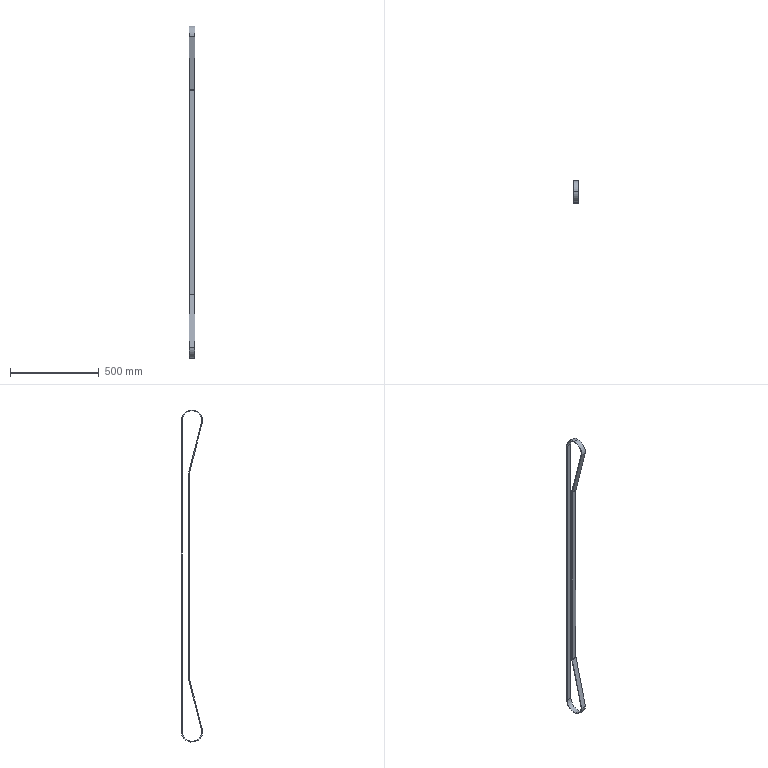Part | SolidWorks | features ExtruThin 1 | 1 solid | 20 faces | box 30 x 121.59 x 1872 mm | volume 524754 mm3 | cylinder 10 | plane 10 | commonest cylinder face diameters 112.59 x3 121.59 x3 37 x2 46 x2
STEP:
#1=CARTESIAN_POINT('',(15.,56.295,1750.));
#2=VERTEX_POINT('',#1);
#3=CARTESIAN_POINT('',(15.,0.,1806.295));
#4=VERTEX_POINT('',#3);
#5=CARTESIAN_POINT('',(15.,0.,1750.));
#6=DIRECTION('',(1.,0.,0.));
#7=DIRECTION('',(0.,0.,-1.));
#8=AXIS2_PLACEMENT_3D('',#5,#6,#7);
#9=CIRCLE('',#8,56.295);
#10=EDGE_CURVE('',#2,#4,#9,.T.);
#11=ORIENTED_EDGE('',*,*,#10,.T.);
#12=CARTESIAN_POINT('',(-15.,0.,1806.295));
#13=VERTEX_POINT('',#12);
#14=CARTESIAN_POINT('',(15.,0.,1806.295));
#15=DIRECTION('',(-1.,0.,0.));
#16=VECTOR('',#15,1000.);
#17=LINE('',#14,#16);
#18=EDGE_CURVE('',#4,#13,#17,.T.);
#19=ORIENTED_EDGE('',*,*,#18,.T.);
#20=CARTESIAN_POINT('',(-15.,56.295,1750.));
#21=VERTEX_POINT('',#20);
#22=CARTESIAN_POINT('',(-15.,0.,1750.));
#23=DIRECTION('',(1.,0.,0.));
#24=DIRECTION('',(0.,0.,-1.));
#25=AXIS2_PLACEMENT_3D('',#22,#23,#24);
#26=CIRCLE('',#25,56.295);
#27=EDGE_CURVE('',#21,#13,#26,.T.);
#28=ORIENTED_EDGE('',*,*,#27,.F.);
#29=CARTESIAN_POINT('',(15.,56.295,1750.));
#30=DIRECTION('',(-1.,0.,0.));
#31=VECTOR('',#30,1000.);
#32=LINE('',#29,#31);
#33=EDGE_CURVE('',#2,#21,#32,.T.);
#34=ORIENTED_EDGE('',*,*,#33,.F.);
#35=EDGE_LOOP('',(#11,#19,#28,#34));
#36=FACE_OUTER_BOUND('',#35,.T.);
#37=CARTESIAN_POINT('',(15.,0.,1750.));
#38=DIRECTION('',(-1.,0.,0.));
#39=DIRECTION('',(0.,0.,1.));
#40=AXIS2_PLACEMENT_3D('',#37,#38,#39);
#41=CYLINDRICAL_SURFACE('',#40,56.295);
#42=ADVANCED_FACE('',(#36),#41,.F.);
#43=CARTESIAN_POINT('',(15.,0.,1810.795));
#44=VERTEX_POINT('',#43);
#45=CARTESIAN_POINT('',(15.,-60.793,1749.552));
#46=VERTEX_POINT('',#45);
#47=CARTESIAN_POINT('',(15.,0.,1750.));
#48=DIRECTION('',(1.,0.,0.));
#49=DIRECTION('',(0.,0.,-1.));
#50=AXIS2_PLACEMENT_3D('',#47,#48,#49);
#51=CIRCLE('',#50,60.795);
#52=EDGE_CURVE('',#44,#46,#51,.T.);
#53=ORIENTED_EDGE('',*,*,#52,.F.);
#54=CARTESIAN_POINT('',(-15.,0.,1810.795));
#55=VERTEX_POINT('',#54);
#56=CARTESIAN_POINT('',(15.,0.,1810.795));
#57=DIRECTION('',(-1.,0.,0.));
#58=VECTOR('',#57,1000.);
#59=LINE('',#56,#58);
#60=EDGE_CURVE('',#44,#55,#59,.T.);
#61=ORIENTED_EDGE('',*,*,#60,.T.);
#62=CARTESIAN_POINT('',(-15.,-60.793,1749.552));
#63=VERTEX_POINT('',#62);
#64=CARTESIAN_POINT('',(-15.,0.,1750.));
#65=DIRECTION('',(1.,0.,0.));
#66=DIRECTION('',(0.,0.,-1.));
#67=AXIS2_PLACEMENT_3D('',#64,#65,#66);
#68=CIRCLE('',#67,60.795);
#69=EDGE_CURVE('',#55,#63,#68,.T.);
#70=ORIENTED_EDGE('',*,*,#69,.T.);
#71=CARTESIAN_POINT('',(15.,-60.793,1749.552));
#72=DIRECTION('',(-1.,0.,0.));
#73=VECTOR('',#72,1000.);
#74=LINE('',#71,#73);
#75=EDGE_CURVE('',#46,#63,#74,.T.);
#76=ORIENTED_EDGE('',*,*,#75,.F.);
#77=EDGE_LOOP('',(#53,#61,#70,#76));
#78=FACE_OUTER_BOUND('',#77,.T.);
#79=CARTESIAN_POINT('',(15.,0.,1750.));
#80=DIRECTION('',(-1.,0.,0.));
#81=DIRECTION('',(0.,0.,1.));
#82=AXIS2_PLACEMENT_3D('',#79,#80,#81);
#83=CYLINDRICAL_SURFACE('',#82,60.795);
#84=ADVANCED_FACE('',(#78),#83,.T.);
#85=CARTESIAN_POINT('',(15.,60.795,1750.));
#86=VERTEX_POINT('',#85);
#87=CARTESIAN_POINT('',(15.,0.,1750.));
#88=DIRECTION('',(1.,0.,0.));
#89=DIRECTION('',(0.,0.,-1.));
#90=AXIS2_PLACEMENT_3D('',#87,#88,#89);
#91=CIRCLE('',#90,60.795);
#92=EDGE_CURVE('',#86,#44,#91,.T.);
#93=ORIENTED_EDGE('',*,*,#92,.T.);
#94=ORIENTED_EDGE('',*,*,#52,.T.);
#95=CARTESIAN_POINT('',(15.,14.914,1454.599));
#96=VERTEX_POINT('',#95);
#97=CARTESIAN_POINT('',(15.,14.914,1454.599));
#98=DIRECTION('',(0.,0.2486,-0.9686));
#99=VECTOR('',#98,1000.);
#100=LINE('',#97,#99);
#101=EDGE_CURVE('',#46,#96,#100,.T.);
#102=ORIENTED_EDGE('',*,*,#101,.T.);
#103=CARTESIAN_POINT('',(15.,15.495,1450.));
#104=VERTEX_POINT('',#103);
#105=CARTESIAN_POINT('',(15.,-3.005,1450.));
#106=DIRECTION('',(-1.,0.,0.));
#107=DIRECTION('',(0.,0.,-1.));
#108=AXIS2_PLACEMENT_3D('',#105,#106,#107);
#109=CIRCLE('',#108,18.5);
#110=EDGE_CURVE('',#96,#104,#109,.T.);
#111=ORIENTED_EDGE('',*,*,#110,.T.);
#112=CARTESIAN_POINT('',(15.,15.495,300.));
#113=VERTEX_POINT('',#112);
#114=CARTESIAN_POINT('',(15.,15.495,1450.));
#115=DIRECTION('',(0.,0.,-1.));
#116=VECTOR('',#115,1000.);
#117=LINE('',#114,#116);
#118=EDGE_CURVE('',#104,#113,#117,.T.);
#119=ORIENTED_EDGE('',*,*,#118,.T.);
#120=CARTESIAN_POINT('',(15.,14.914,295.401));
#121=VERTEX_POINT('',#120);
#122=CARTESIAN_POINT('',(15.,-3.005,300.));
#123=DIRECTION('',(-1.,0.,0.));
#124=DIRECTION('',(0.,0.,-1.));
#125=AXIS2_PLACEMENT_3D('',#122,#123,#124);
#126=CIRCLE('',#125,18.5);
#127=EDGE_CURVE('',#113,#121,#126,.T.);
#128=ORIENTED_EDGE('',*,*,#127,.T.);
#129=CARTESIAN_POINT('',(15.,-60.793,0.4485));
#130=VERTEX_POINT('',#129);
#131=CARTESIAN_POINT('',(15.,-60.685,0.8702));
#132=DIRECTION('',(0.,-0.2486,-0.9686));
#133=VECTOR('',#132,1000.);
#134=LINE('',#131,#133);
#135=EDGE_CURVE('',#121,#130,#134,.T.);
#136=ORIENTED_EDGE('',*,*,#135,.T.);
#137=CARTESIAN_POINT('',(15.,60.795,0.));
#138=VERTEX_POINT('',#137);
#139=CARTESIAN_POINT('',(15.,0.,0.));
#140=DIRECTION('',(1.,0.,0.));
#141=DIRECTION('',(0.,0.,-1.));
#142=AXIS2_PLACEMENT_3D('',#139,#140,#141);
#143=CIRCLE('',#142,60.795);
#144=EDGE_CURVE('',#130,#138,#143,.T.);
#145=ORIENTED_EDGE('',*,*,#144,.T.);
#146=CARTESIAN_POINT('',(15.,60.795,0.));
#147=DIRECTION('',(0.,0.,1.));
#148=VECTOR('',#147,1000.);
#149=LINE('',#146,#148);
#150=EDGE_CURVE('',#138,#86,#149,.T.);
#151=ORIENTED_EDGE('',*,*,#150,.T.);
#152=EDGE_LOOP('',(#93,#94,#102,#111,#119,#128,#136,#145,#151));
#153=FACE_OUTER_BOUND('',#152,.T.);
#154=CARTESIAN_POINT('',(15.,-56.295,1750.126));
#155=VERTEX_POINT('',#154);
#156=CARTESIAN_POINT('',(15.,19.273,1455.718));
#157=VERTEX_POINT('',#156);
#158=CARTESIAN_POINT('',(15.,19.273,1455.718));
#159=DIRECTION('',(0.,0.2486,-0.9686));
#160=VECTOR('',#159,1000.);
#161=LINE('',#158,#160);
#162=EDGE_CURVE('',#155,#157,#161,.T.);
#163=ORIENTED_EDGE('',*,*,#162,.F.);
#164=CARTESIAN_POINT('',(15.,0.,1750.));
#165=DIRECTION('',(1.,0.,0.));
#166=DIRECTION('',(0.,0.,-1.));
#167=AXIS2_PLACEMENT_3D('',#164,#165,#166);
#168=CIRCLE('',#167,56.295);
#169=EDGE_CURVE('',#4,#155,#168,.T.);
#170=ORIENTED_EDGE('',*,*,#169,.F.);
#171=ORIENTED_EDGE('',*,*,#10,.F.);
#172=CARTESIAN_POINT('',(15.,56.295,0.));
#173=VERTEX_POINT('',#172);
#174=CARTESIAN_POINT('',(15.,56.295,0.));
#175=DIRECTION('',(0.,0.,1.));
#176=VECTOR('',#175,1000.);
#177=LINE('',#174,#176);
#178=EDGE_CURVE('',#173,#2,#177,.T.);
#179=ORIENTED_EDGE('',*,*,#178,.F.);
#180=CARTESIAN_POINT('',(15.,-56.295,-0.1257));
#181=VERTEX_POINT('',#180);
#182=CARTESIAN_POINT('',(15.,0.,0.));
#183=DIRECTION('',(1.,0.,0.));
#184=DIRECTION('',(0.,0.,-1.));
#185=AXIS2_PLACEMENT_3D('',#182,#183,#184);
#186=CIRCLE('',#185,56.295);
#187=EDGE_CURVE('',#181,#173,#186,.T.);
#188=ORIENTED_EDGE('',*,*,#187,.F.);
#189=CARTESIAN_POINT('',(15.,19.273,294.282));
#190=VERTEX_POINT('',#189);
#191=CARTESIAN_POINT('',(15.,-56.326,-0.2486));
#192=DIRECTION('',(0.,-0.2486,-0.9686));
#193=VECTOR('',#192,1000.);
#194=LINE('',#191,#193);
#195=EDGE_CURVE('',#190,#181,#194,.T.);
#196=ORIENTED_EDGE('',*,*,#195,.F.);
#197=CARTESIAN_POINT('',(15.,19.995,300.));
#198=VERTEX_POINT('',#197);
#199=CARTESIAN_POINT('',(15.,-3.005,300.));
#200=DIRECTION('',(-1.,0.,0.));
#201=DIRECTION('',(0.,0.,-1.));
#202=AXIS2_PLACEMENT_3D('',#199,#200,#201);
#203=CIRCLE('',#202,23.);
#204=EDGE_CURVE('',#198,#190,#203,.T.);
#205=ORIENTED_EDGE('',*,*,#204,.F.);
#206=CARTESIAN_POINT('',(15.,19.995,1450.));
#207=VERTEX_POINT('',#206);
#208=CARTESIAN_POINT('',(15.,19.995,1450.));
#209=DIRECTION('',(0.,0.,-1.));
#210=VECTOR('',#209,1000.);
#211=LINE('',#208,#210);
#212=EDGE_CURVE('',#207,#198,#211,.T.);
#213=ORIENTED_EDGE('',*,*,#212,.F.);
#214=CARTESIAN_POINT('',(15.,-3.005,1450.));
#215=DIRECTION('',(-1.,0.,0.));
#216=DIRECTION('',(0.,0.,-1.));
#217=AXIS2_PLACEMENT_3D('',#214,#215,#216);
#218=CIRCLE('',#217,23.);
#219=EDGE_CURVE('',#157,#207,#218,.T.);
#220=ORIENTED_EDGE('',*,*,#219,.F.);
#221=EDGE_LOOP('',(#163,#170,#171,#179,#188,#196,#205,#213,#220));
#222=FACE_BOUND('',#221,.T.);
#223=CARTESIAN_POINT('',(15.,0.,1750.));
#224=DIRECTION('',(1.,0.,0.));
#225=DIRECTION('',(0.,0.,-1.));
#226=AXIS2_PLACEMENT_3D('',#223,#224,#225);
#227=PLANE('',#226);
#228=ADVANCED_FACE('',(#153,#222),#227,.T.);
#229=CARTESIAN_POINT('',(-15.,60.795,1750.));
#230=VERTEX_POINT('',#229);
#231=CARTESIAN_POINT('',(-15.,0.,1750.));
#232=DIRECTION('',(1.,0.,0.));
#233=DIRECTION('',(0.,0.,-1.));
#234=AXIS2_PLACEMENT_3D('',#231,#232,#233);
#235=CIRCLE('',#234,60.795);
#236=EDGE_CURVE('',#230,#55,#235,.T.);
#237=ORIENTED_EDGE('',*,*,#236,.F.);
#238=CARTESIAN_POINT('',(-15.,60.795,0.));
#239=VERTEX_POINT('',#238);
#240=CARTESIAN_POINT('',(-15.,60.795,0.));
#241=DIRECTION('',(0.,0.,1.));
#242=VECTOR('',#241,1000.);
#243=LINE('',#240,#242);
#244=EDGE_CURVE('',#239,#230,#243,.T.);
#245=ORIENTED_EDGE('',*,*,#244,.F.);
#246=CARTESIAN_POINT('',(-15.,-60.793,0.4485));
#247=VERTEX_POINT('',#246);
#248=CARTESIAN_POINT('',(-15.,0.,0.));
#249=DIRECTION('',(1.,0.,0.));
#250=DIRECTION('',(0.,0.,-1.));
#251=AXIS2_PLACEMENT_3D('',#248,#249,#250);
#252=CIRCLE('',#251,60.795);
#253=EDGE_CURVE('',#247,#239,#252,.T.);
#254=ORIENTED_EDGE('',*,*,#253,.F.);
#255=CARTESIAN_POINT('',(-15.,14.914,295.401));
#256=VERTEX_POINT('',#255);
#257=CARTESIAN_POINT('',(-15.,-60.685,0.8702));
#258=DIRECTION('',(0.,-0.2486,-0.9686));
#259=VECTOR('',#258,1000.);
#260=LINE('',#257,#259);
#261=EDGE_CURVE('',#256,#247,#260,.T.);
#262=ORIENTED_EDGE('',*,*,#261,.F.);
#263=CARTESIAN_POINT('',(-15.,15.495,300.));
#264=VERTEX_POINT('',#263);
#265=CARTESIAN_POINT('',(-15.,-3.005,300.));
#266=DIRECTION('',(-1.,0.,0.));
#267=DIRECTION('',(0.,0.,-1.));
#268=AXIS2_PLACEMENT_3D('',#265,#266,#267);
#269=CIRCLE('',#268,18.5);
#270=EDGE_CURVE('',#264,#256,#269,.T.);
#271=ORIENTED_EDGE('',*,*,#270,.F.);
#272=CARTESIAN_POINT('',(-15.,15.495,1450.));
#273=VERTEX_POINT('',#272);
#274=CARTESIAN_POINT('',(-15.,15.495,1450.));
#275=DIRECTION('',(0.,0.,-1.));
#276=VECTOR('',#275,1000.);
#277=LINE('',#274,#276);
#278=EDGE_CURVE('',#273,#264,#277,.T.);
#279=ORIENTED_EDGE('',*,*,#278,.F.);
#280=CARTESIAN_POINT('',(-15.,14.914,1454.599));
#281=VERTEX_POINT('',#280);
#282=CARTESIAN_POINT('',(-15.,-3.005,1450.));
#283=DIRECTION('',(-1.,0.,0.));
#284=DIRECTION('',(0.,0.,-1.));
#285=AXIS2_PLACEMENT_3D('',#282,#283,#284);
#286=CIRCLE('',#285,18.5);
#287=EDGE_CURVE('',#281,#273,#286,.T.);
#288=ORIENTED_EDGE('',*,*,#287,.F.);
#289=CARTESIAN_POINT('',(-15.,14.914,1454.599));
#290=DIRECTION('',(0.,0.2486,-0.9686));
#291=VECTOR('',#290,1000.);
#292=LINE('',#289,#291);
#293=EDGE_CURVE('',#63,#281,#292,.T.);
#294=ORIENTED_EDGE('',*,*,#293,.F.);
#295=ORIENTED_EDGE('',*,*,#69,.F.);
#296=EDGE_LOOP('',(#237,#245,#254,#262,#271,#279,#288,#294,#295));
#297=FACE_OUTER_BOUND('',#296,.T.);
#298=ORIENTED_EDGE('',*,*,#27,.T.);
#299=CARTESIAN_POINT('',(-15.,-56.295,1750.126));
#300=VERTEX_POINT('',#299);
#301=CARTESIAN_POINT('',(-15.,0.,1750.));
#302=DIRECTION('',(1.,0.,0.));
#303=DIRECTION('',(0.,0.,-1.));
#304=AXIS2_PLACEMENT_3D('',#301,#302,#303);
#305=CIRCLE('',#304,56.295);
#306=EDGE_CURVE('',#13,#300,#305,.T.);
#307=ORIENTED_EDGE('',*,*,#306,.T.);
#308=CARTESIAN_POINT('',(-15.,19.273,1455.718));
#309=VERTEX_POINT('',#308);
#310=CARTESIAN_POINT('',(-15.,19.273,1455.718));
#311=DIRECTION('',(0.,0.2486,-0.9686));
#312=VECTOR('',#311,1000.);
#313=LINE('',#310,#312);
#314=EDGE_CURVE('',#300,#309,#313,.T.);
#315=ORIENTED_EDGE('',*,*,#314,.T.);
#316=CARTESIAN_POINT('',(-15.,19.995,1450.));
#317=VERTEX_POINT('',#316);
#318=CARTESIAN_POINT('',(-15.,-3.005,1450.));
#319=DIRECTION('',(-1.,0.,0.));
#320=DIRECTION('',(0.,0.,-1.));
#321=AXIS2_PLACEMENT_3D('',#318,#319,#320);
#322=CIRCLE('',#321,23.);
#323=EDGE_CURVE('',#309,#317,#322,.T.);
#324=ORIENTED_EDGE('',*,*,#323,.T.);
#325=CARTESIAN_POINT('',(-15.,19.995,300.));
#326=VERTEX_POINT('',#325);
#327=CARTESIAN_POINT('',(-15.,19.995,1450.));
#328=DIRECTION('',(0.,0.,-1.));
#329=VECTOR('',#328,1000.);
#330=LINE('',#327,#329);
#331=EDGE_CURVE('',#317,#326,#330,.T.);
#332=ORIENTED_EDGE('',*,*,#331,.T.);
#333=CARTESIAN_POINT('',(-15.,19.273,294.282));
#334=VERTEX_POINT('',#333);
#335=CARTESIAN_POINT('',(-15.,-3.005,300.));
#336=DIRECTION('',(-1.,0.,0.));
#337=DIRECTION('',(0.,0.,-1.));
#338=AXIS2_PLACEMENT_3D('',#335,#336,#337);
#339=CIRCLE('',#338,23.);
#340=EDGE_CURVE('',#326,#334,#339,.T.);
#341=ORIENTED_EDGE('',*,*,#340,.T.);
#342=CARTESIAN_POINT('',(-15.,-56.295,-0.1257));
#343=VERTEX_POINT('',#342);
#344=CARTESIAN_POINT('',(-15.,-56.326,-0.2486));
#345=DIRECTION('',(0.,-0.2486,-0.9686));
#346=VECTOR('',#345,1000.);
#347=LINE('',#344,#346);
#348=EDGE_CURVE('',#334,#343,#347,.T.);
#349=ORIENTED_EDGE('',*,*,#348,.T.);
#350=CARTESIAN_POINT('',(-15.,56.295,0.));
#351=VERTEX_POINT('',#350);
#352=CARTESIAN_POINT('',(-15.,0.,0.));
#353=DIRECTION('',(1.,0.,0.));
#354=DIRECTION('',(0.,0.,-1.));
#355=AXIS2_PLACEMENT_3D('',#352,#353,#354);
#356=CIRCLE('',#355,56.295);
#357=EDGE_CURVE('',#343,#351,#356,.T.);
#358=ORIENTED_EDGE('',*,*,#357,.T.);
#359=CARTESIAN_POINT('',(-15.,56.295,0.));
#360=DIRECTION('',(0.,0.,1.));
#361=VECTOR('',#360,1000.);
#362=LINE('',#359,#361);
#363=EDGE_CURVE('',#351,#21,#362,.T.);
#364=ORIENTED_EDGE('',*,*,#363,.T.);
#365=EDGE_LOOP('',(#298,#307,#315,#324,#332,#341,#349,#358,#364));
#366=FACE_BOUND('',#365,.T.);
#367=CARTESIAN_POINT('',(-15.,0.,1750.));
#368=DIRECTION('',(1.,0.,0.));
#369=DIRECTION('',(0.,0.,-1.));
#370=AXIS2_PLACEMENT_3D('',#367,#368,#369);
#371=PLANE('',#370);
#372=ADVANCED_FACE('',(#297,#366),#371,.F.);
#373=ORIENTED_EDGE('',*,*,#60,.F.);
#374=ORIENTED_EDGE('',*,*,#92,.F.);
#375=CARTESIAN_POINT('',(15.,60.795,1750.));
#376=DIRECTION('',(-1.,0.,0.));
#377=VECTOR('',#376,1000.);
#378=LINE('',#375,#377);
#379=EDGE_CURVE('',#86,#230,#378,.T.);
#380=ORIENTED_EDGE('',*,*,#379,.T.);
#381=ORIENTED_EDGE('',*,*,#236,.T.);
#382=EDGE_LOOP('',(#373,#374,#380,#381));
#383=FACE_OUTER_BOUND('',#382,.T.);
#384=CARTESIAN_POINT('',(15.,0.,1750.));
#385=DIRECTION('',(-1.,0.,0.));
#386=DIRECTION('',(0.,0.,1.));
#387=AXIS2_PLACEMENT_3D('',#384,#385,#386);
#388=CYLINDRICAL_SURFACE('',#387,60.795);
#389=ADVANCED_FACE('',(#383),#388,.T.);
#390=ORIENTED_EDGE('',*,*,#293,.T.);
#391=CARTESIAN_POINT('',(15.,14.914,1454.599));
#392=DIRECTION('',(-1.,0.,0.));
#393=VECTOR('',#392,1000.);
#394=LINE('',#391,#393);
#395=EDGE_CURVE('',#96,#281,#394,.T.);
#396=ORIENTED_EDGE('',*,*,#395,.F.);
#397=ORIENTED_EDGE('',*,*,#101,.F.);
#398=ORIENTED_EDGE('',*,*,#75,.T.);
#399=EDGE_LOOP('',(#390,#396,#397,#398));
#400=FACE_OUTER_BOUND('',#399,.T.);
#401=CARTESIAN_POINT('',(15.,14.914,1454.599));
#402=DIRECTION('',(0.,0.9686,0.2486));
#403=DIRECTION('',(0.,-0.2486,0.9686));
#404=AXIS2_PLACEMENT_3D('',#401,#402,#403);
#405=PLANE('',#404);
#406=ADVANCED_FACE('',(#400),#405,.F.);
#407=ORIENTED_EDGE('',*,*,#287,.T.);
#408=CARTESIAN_POINT('',(15.,15.495,1450.));
#409=DIRECTION('',(-1.,0.,0.));
#410=VECTOR('',#409,1000.);
#411=LINE('',#408,#410);
#412=EDGE_CURVE('',#104,#273,#411,.T.);
#413=ORIENTED_EDGE('',*,*,#412,.F.);
#414=ORIENTED_EDGE('',*,*,#110,.F.);
#415=ORIENTED_EDGE('',*,*,#395,.T.);
#416=EDGE_LOOP('',(#407,#413,#414,#415));
#417=FACE_OUTER_BOUND('',#416,.T.);
#418=CARTESIAN_POINT('',(15.,-3.005,1450.));
#419=DIRECTION('',(-1.,0.,0.));
#420=DIRECTION('',(0.,0.,1.));
#421=AXIS2_PLACEMENT_3D('',#418,#419,#420);
#422=CYLINDRICAL_SURFACE('',#421,18.5);
#423=ADVANCED_FACE('',(#417),#422,.F.);
#424=ORIENTED_EDGE('',*,*,#278,.T.);
#425=CARTESIAN_POINT('',(15.,15.495,300.));
#426=DIRECTION('',(-1.,0.,0.));
#427=VECTOR('',#426,1000.);
#428=LINE('',#425,#427);
#429=EDGE_CURVE('',#113,#264,#428,.T.);
#430=ORIENTED_EDGE('',*,*,#429,.F.);
#431=ORIENTED_EDGE('',*,*,#118,.F.);
#432=ORIENTED_EDGE('',*,*,#412,.T.);
#433=EDGE_LOOP('',(#424,#430,#431,#432));
#434=FACE_OUTER_BOUND('',#433,.T.);
#435=CARTESIAN_POINT('',(15.,15.495,1450.));
#436=DIRECTION('',(0.,1.,0.));
#437=DIRECTION('',(0.,0.,1.));
#438=AXIS2_PLACEMENT_3D('',#435,#436,#437);
#439=PLANE('',#438);
#440=ADVANCED_FACE('',(#434),#439,.F.);
#441=ORIENTED_EDGE('',*,*,#270,.T.);
#442=CARTESIAN_POINT('',(15.,14.914,295.401));
#443=DIRECTION('',(-1.,0.,0.));
#444=VECTOR('',#443,1000.);
#445=LINE('',#442,#444);
#446=EDGE_CURVE('',#121,#256,#445,.T.);
#447=ORIENTED_EDGE('',*,*,#446,.F.);
#448=ORIENTED_EDGE('',*,*,#127,.F.);
#449=ORIENTED_EDGE('',*,*,#429,.T.);
#450=EDGE_LOOP('',(#441,#447,#448,#449));
#451=FACE_OUTER_BOUND('',#450,.T.);
#452=CARTESIAN_POINT('',(15.,-3.005,300.));
#453=DIRECTION('',(-1.,0.,0.));
#454=DIRECTION('',(0.,0.,1.));
#455=AXIS2_PLACEMENT_3D('',#452,#453,#454);
#456=CYLINDRICAL_SURFACE('',#455,18.5);
#457=ADVANCED_FACE('',(#451),#456,.F.);
#458=ORIENTED_EDGE('',*,*,#261,.T.);
#459=CARTESIAN_POINT('',(15.,-60.793,0.4485));
#460=DIRECTION('',(-1.,0.,0.));
#461=VECTOR('',#460,1000.);
#462=LINE('',#459,#461);
#463=EDGE_CURVE('',#130,#247,#462,.T.);
#464=ORIENTED_EDGE('',*,*,#463,.F.);
#465=ORIENTED_EDGE('',*,*,#135,.F.);
#466=ORIENTED_EDGE('',*,*,#446,.T.);
#467=EDGE_LOOP('',(#458,#464,#465,#466));
#468=FACE_OUTER_BOUND('',#467,.T.);
#469=CARTESIAN_POINT('',(15.,-60.685,0.8702));
#470=DIRECTION('',(0.,0.9686,-0.2486));
#471=DIRECTION('',(0.,0.2486,0.9686));
#472=AXIS2_PLACEMENT_3D('',#469,#470,#471);
#473=PLANE('',#472);
#474=ADVANCED_FACE('',(#468),#473,.F.);
#475=ORIENTED_EDGE('',*,*,#253,.T.);
#476=CARTESIAN_POINT('',(15.,60.795,0.));
#477=DIRECTION('',(-1.,0.,0.));
#478=VECTOR('',#477,1000.);
#479=LINE('',#476,#478);
#480=EDGE_CURVE('',#138,#239,#479,.T.);
#481=ORIENTED_EDGE('',*,*,#480,.F.);
#482=ORIENTED_EDGE('',*,*,#144,.F.);
#483=ORIENTED_EDGE('',*,*,#463,.T.);
#484=EDGE_LOOP('',(#475,#481,#482,#483));
#485=FACE_OUTER_BOUND('',#484,.T.);
#486=CARTESIAN_POINT('',(15.,0.,0.));
#487=DIRECTION('',(-1.,0.,0.));
#488=DIRECTION('',(0.,0.,1.));
#489=AXIS2_PLACEMENT_3D('',#486,#487,#488);
#490=CYLINDRICAL_SURFACE('',#489,60.795);
#491=ADVANCED_FACE('',(#485),#490,.T.);
#492=ORIENTED_EDGE('',*,*,#244,.T.);
#493=ORIENTED_EDGE('',*,*,#379,.F.);
#494=ORIENTED_EDGE('',*,*,#150,.F.);
#495=ORIENTED_EDGE('',*,*,#480,.T.);
#496=EDGE_LOOP('',(#492,#493,#494,#495));
#497=FACE_OUTER_BOUND('',#496,.T.);
#498=CARTESIAN_POINT('',(15.,60.795,0.));
#499=DIRECTION('',(0.,-1.,0.));
#500=DIRECTION('',(0.,0.,-1.));
#501=AXIS2_PLACEMENT_3D('',#498,#499,#500);
#502=PLANE('',#501);
#503=ADVANCED_FACE('',(#497),#502,.F.);
#504=ORIENTED_EDGE('',*,*,#18,.F.);
#505=ORIENTED_EDGE('',*,*,#169,.T.);
#506=CARTESIAN_POINT('',(15.,-56.295,1750.126));
#507=DIRECTION('',(-1.,0.,0.));
#508=VECTOR('',#507,1000.);
#509=LINE('',#506,#508);
#510=EDGE_CURVE('',#155,#300,#509,.T.);
#511=ORIENTED_EDGE('',*,*,#510,.T.);
#512=ORIENTED_EDGE('',*,*,#306,.F.);
#513=EDGE_LOOP('',(#504,#505,#511,#512));
#514=FACE_OUTER_BOUND('',#513,.T.);
#515=CARTESIAN_POINT('',(15.,0.,1750.));
#516=DIRECTION('',(-1.,0.,0.));
#517=DIRECTION('',(0.,0.,1.));
#518=AXIS2_PLACEMENT_3D('',#515,#516,#517);
#519=CYLINDRICAL_SURFACE('',#518,56.295);
#520=ADVANCED_FACE('',(#514),#519,.F.);
#521=ORIENTED_EDGE('',*,*,#314,.F.);
#522=ORIENTED_EDGE('',*,*,#510,.F.);
#523=ORIENTED_EDGE('',*,*,#162,.T.);
#524=CARTESIAN_POINT('',(15.,19.273,1455.718));
#525=DIRECTION('',(-1.,0.,0.));
#526=VECTOR('',#525,1000.);
#527=LINE('',#524,#526);
#528=EDGE_CURVE('',#157,#309,#527,.T.);
#529=ORIENTED_EDGE('',*,*,#528,.T.);
#530=EDGE_LOOP('',(#521,#522,#523,#529));
#531=FACE_OUTER_BOUND('',#530,.T.);
#532=CARTESIAN_POINT('',(15.,19.273,1455.718));
#533=DIRECTION('',(0.,0.9686,0.2486));
#534=DIRECTION('',(0.,-0.2486,0.9686));
#535=AXIS2_PLACEMENT_3D('',#532,#533,#534);
#536=PLANE('',#535);
#537=ADVANCED_FACE('',(#531),#536,.T.);
#538=ORIENTED_EDGE('',*,*,#323,.F.);
#539=ORIENTED_EDGE('',*,*,#528,.F.);
#540=ORIENTED_EDGE('',*,*,#219,.T.);
#541=CARTESIAN_POINT('',(15.,19.995,1450.));
#542=DIRECTION('',(-1.,0.,0.));
#543=VECTOR('',#542,1000.);
#544=LINE('',#541,#543);
#545=EDGE_CURVE('',#207,#317,#544,.T.);
#546=ORIENTED_EDGE('',*,*,#545,.T.);
#547=EDGE_LOOP('',(#538,#539,#540,#546));
#548=FACE_OUTER_BOUND('',#547,.T.);
#549=CARTESIAN_POINT('',(15.,-3.005,1450.));
#550=DIRECTION('',(-1.,0.,0.));
#551=DIRECTION('',(0.,0.,1.));
#552=AXIS2_PLACEMENT_3D('',#549,#550,#551);
#553=CYLINDRICAL_SURFACE('',#552,23.);
#554=ADVANCED_FACE('',(#548),#553,.T.);
#555=ORIENTED_EDGE('',*,*,#331,.F.);
#556=ORIENTED_EDGE('',*,*,#545,.F.);
#557=ORIENTED_EDGE('',*,*,#212,.T.);
#558=CARTESIAN_POINT('',(15.,19.995,300.));
#559=DIRECTION('',(-1.,0.,0.));
#560=VECTOR('',#559,1000.);
#561=LINE('',#558,#560);
#562=EDGE_CURVE('',#198,#326,#561,.T.);
#563=ORIENTED_EDGE('',*,*,#562,.T.);
#564=EDGE_LOOP('',(#555,#556,#557,#563));
#565=FACE_OUTER_BOUND('',#564,.T.);
#566=CARTESIAN_POINT('',(15.,19.995,1450.));
#567=DIRECTION('',(0.,1.,0.));
#568=DIRECTION('',(0.,0.,1.));
#569=AXIS2_PLACEMENT_3D('',#566,#567,#568);
#570=PLANE('',#569);
#571=ADVANCED_FACE('',(#565),#570,.T.);
#572=ORIENTED_EDGE('',*,*,#340,.F.);
#573=ORIENTED_EDGE('',*,*,#562,.F.);
#574=ORIENTED_EDGE('',*,*,#204,.T.);
#575=CARTESIAN_POINT('',(15.,19.273,294.282));
#576=DIRECTION('',(-1.,0.,0.));
#577=VECTOR('',#576,1000.);
#578=LINE('',#575,#577);
#579=EDGE_CURVE('',#190,#334,#578,.T.);
#580=ORIENTED_EDGE('',*,*,#579,.T.);
#581=EDGE_LOOP('',(#572,#573,#574,#580));
#582=FACE_OUTER_BOUND('',#581,.T.);
#583=CARTESIAN_POINT('',(15.,-3.005,300.));
#584=DIRECTION('',(-1.,0.,0.));
#585=DIRECTION('',(0.,0.,1.));
#586=AXIS2_PLACEMENT_3D('',#583,#584,#585);
#587=CYLINDRICAL_SURFACE('',#586,23.);
#588=ADVANCED_FACE('',(#582),#587,.T.);
#589=ORIENTED_EDGE('',*,*,#348,.F.);
#590=ORIENTED_EDGE('',*,*,#579,.F.);
#591=ORIENTED_EDGE('',*,*,#195,.T.);
#592=CARTESIAN_POINT('',(15.,-56.295,-0.1257));
#593=DIRECTION('',(-1.,0.,0.));
#594=VECTOR('',#593,1000.);
#595=LINE('',#592,#594);
#596=EDGE_CURVE('',#181,#343,#595,.T.);
#597=ORIENTED_EDGE('',*,*,#596,.T.);
#598=EDGE_LOOP('',(#589,#590,#591,#597));
#599=FACE_OUTER_BOUND('',#598,.T.);
#600=CARTESIAN_POINT('',(15.,-56.326,-0.2486));
#601=DIRECTION('',(0.,0.9686,-0.2486));
#602=DIRECTION('',(0.,0.2486,0.9686));
#603=AXIS2_PLACEMENT_3D('',#600,#601,#602);
#604=PLANE('',#603);
#605=ADVANCED_FACE('',(#599),#604,.T.);
#606=ORIENTED_EDGE('',*,*,#357,.F.);
#607=ORIENTED_EDGE('',*,*,#596,.F.);
#608=ORIENTED_EDGE('',*,*,#187,.T.);
#609=CARTESIAN_POINT('',(15.,56.295,0.));
#610=DIRECTION('',(-1.,0.,0.));
#611=VECTOR('',#610,1000.);
#612=LINE('',#609,#611);
#613=EDGE_CURVE('',#173,#351,#612,.T.);
#614=ORIENTED_EDGE('',*,*,#613,.T.);
#615=EDGE_LOOP('',(#606,#607,#608,#614));
#616=FACE_OUTER_BOUND('',#615,.T.);
#617=CARTESIAN_POINT('',(15.,0.,0.));
#618=DIRECTION('',(-1.,0.,0.));
#619=DIRECTION('',(0.,0.,1.));
#620=AXIS2_PLACEMENT_3D('',#617,#618,#619);
#621=CYLINDRICAL_SURFACE('',#620,56.295);
#622=ADVANCED_FACE('',(#616),#621,.F.);
#623=ORIENTED_EDGE('',*,*,#363,.F.);
#624=ORIENTED_EDGE('',*,*,#613,.F.);
#625=ORIENTED_EDGE('',*,*,#178,.T.);
#626=ORIENTED_EDGE('',*,*,#33,.T.);
#627=EDGE_LOOP('',(#623,#624,#625,#626));
#628=FACE_OUTER_BOUND('',#627,.T.);
#629=CARTESIAN_POINT('',(15.,56.295,0.));
#630=DIRECTION('',(0.,-1.,0.));
#631=DIRECTION('',(0.,0.,-1.));
#632=AXIS2_PLACEMENT_3D('',#629,#630,#631);
#633=PLANE('',#632);
#634=ADVANCED_FACE('',(#628),#633,.T.);
#635=CLOSED_SHELL('',(#42,#84,#228,#372,#389,#406,#423,#440,#457,#474,#491,#503,#520,#537,#554,#571,#588,#605,#622,#634));
#636=MANIFOLD_SOLID_BREP('',#635);
#637=CARTESIAN_POINT('',(0.,0.,0.));
#638=DIRECTION('',(0.,0.,1.));
#639=DIRECTION('',(1.,0.,0.));
#640=AXIS2_PLACEMENT_3D('',#637,#638,#639);
#641=(LENGTH_UNIT()NAMED_UNIT(*)SI_UNIT(.MILLI.,.METRE.));
#642=UNCERTAINTY_MEASURE_WITH_UNIT(LENGTH_MEASURE(0.00001),#641,'','');
#643=(NAMED_UNIT(*)PLANE_ANGLE_UNIT()SI_UNIT($,.RADIAN.));
#644=(NAMED_UNIT(*)SI_UNIT($,.STERADIAN.)SOLID_ANGLE_UNIT());
#645=(GEOMETRIC_REPRESENTATION_CONTEXT(3)GLOBAL_UNCERTAINTY_ASSIGNED_CONTEXT((#642))GLOBAL_UNIT_ASSIGNED_CONTEXT((#641,#643,#644))REPRESENTATION_CONTEXT('',''));
#646=ADVANCED_BREP_SHAPE_REPRESENTATION('',(#636,#640),#645);